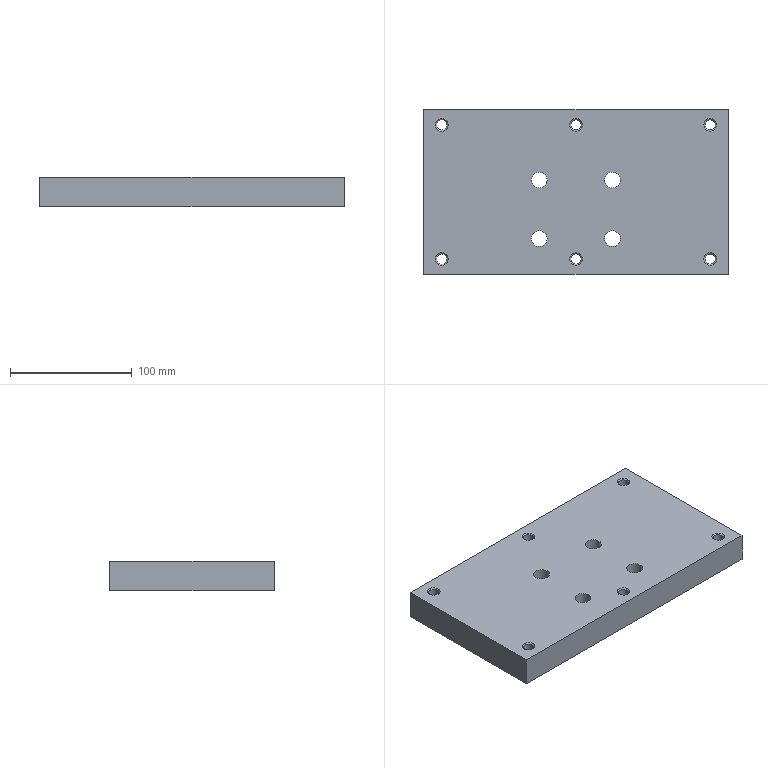Part | STEP file | BAT VOI MANG CA CO LOGO | 1 solid | 72 faces | box 250 x 135 x 24 mm | volume 764464 mm3 | cylinder 36 | cone 22 | plane 14 | commonest cylinder face diameters 8.376 x12 13 x8 18 x8 20 x8